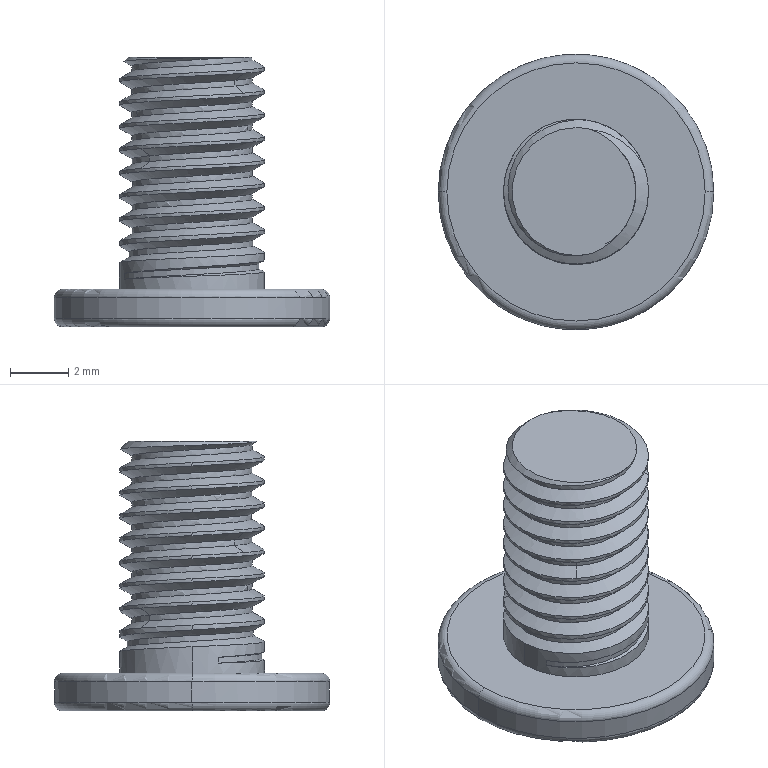Part | NX | features solid 2 | 1 solid | 47 faces | box 9.5 x 9.5 x 9.3 mm | volume 204.641 mm3 | cylinder 20 | spline 12 | plane 10 | torus 4 | cone 1 | commonest cylinder face diameters 5 x18 9.5 x2